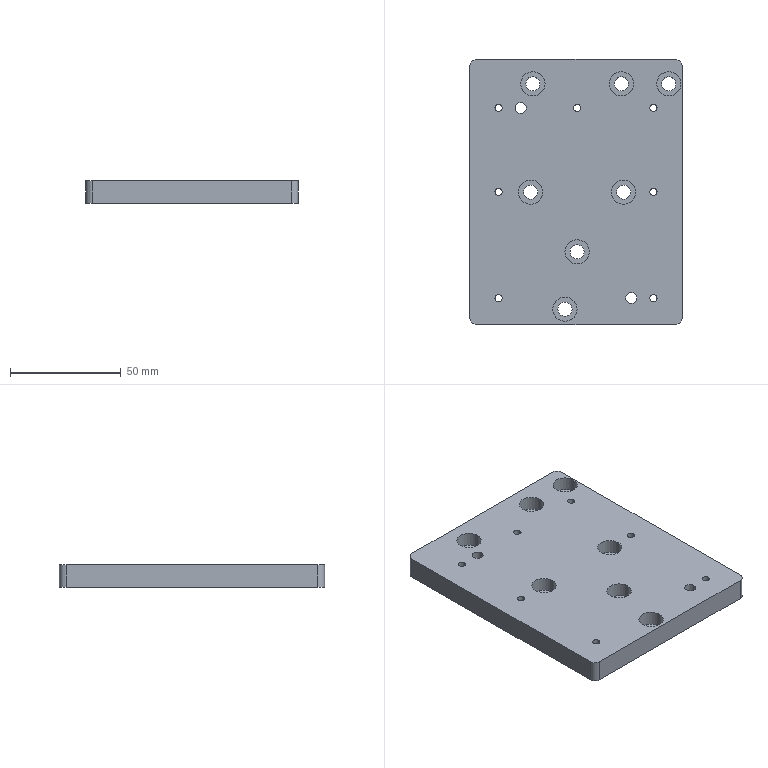Part | SolidWorks | features HoleWzd 2, Extrusion 1, Fillet 1, ICE 1 | 1 solid | 63 faces | box 96 x 120 x 10 mm | volume 109019 mm3 | cylinder 50 | plane 13 | commonest cylinder face diameters 3.3 x14 6.4 x14 11 x14 5 x4 6 x4